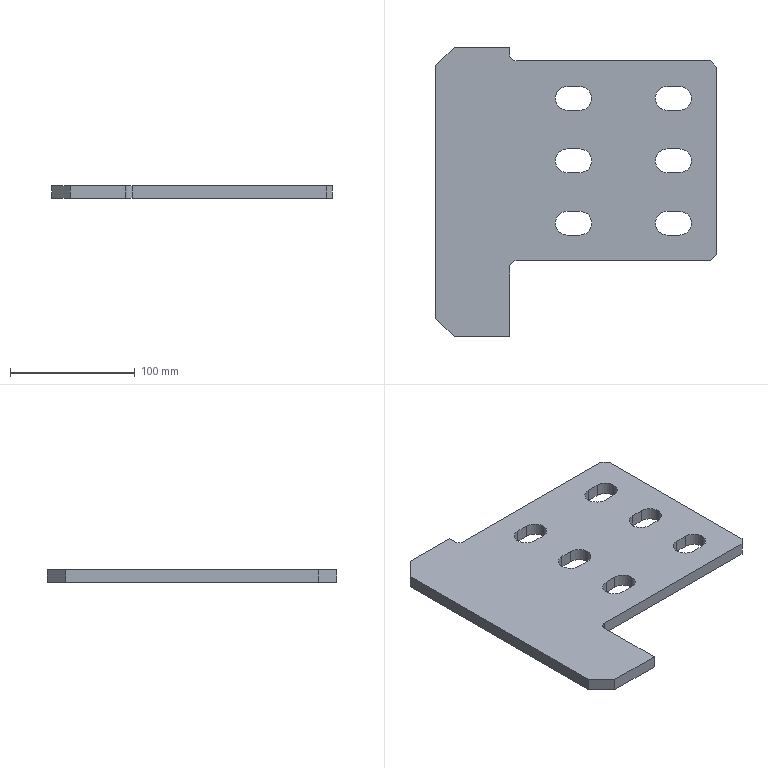Part | STEP file | 筋Plate-250×125-200-60度 | 1 solid | 46 faces | box 225 x 232 x 10 mm | volume 372036 mm3 | plane 26 | cylinder 20 | commonest cylinder face diameters 19 x18 10 x2